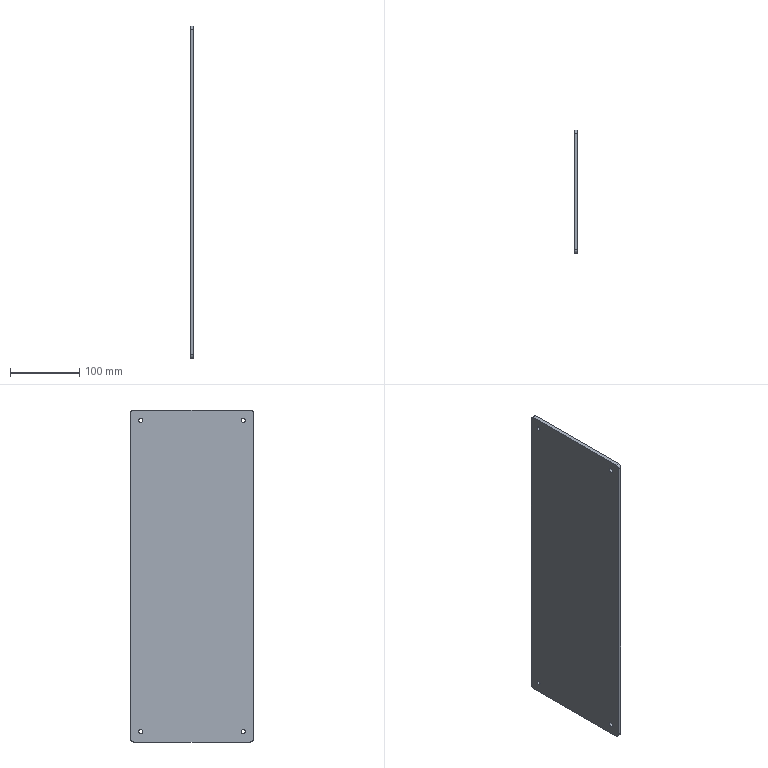Part | SolidWorks | features Extrusion 1, Fillet 1, ICE 1 | 1 solid | 18 faces | box 5 x 178 x 480 mm | volume 426527 mm3 | cylinder 12 | plane 6 | commonest cylinder face diameters 6 x8 10 x4
STEP:
#1=CARTESIAN_POINT('',(0.,-74.,-222.));
#2=VERTEX_POINT('',#1);
#3=CARTESIAN_POINT('',(0.,-74.,-228.));
#4=VERTEX_POINT('',#3);
#5=CARTESIAN_POINT('',(0.,-74.,-225.));
#6=DIRECTION('',(1.,0.,0.));
#7=DIRECTION('',(0.,0.,-1.));
#8=AXIS2_PLACEMENT_3D('',#5,#6,#7);
#9=CIRCLE('',#8,3.);
#10=EDGE_CURVE('',#2,#4,#9,.T.);
#11=ORIENTED_EDGE('',*,*,#10,.F.);
#12=CARTESIAN_POINT('',(5.,-74.,-222.));
#13=VERTEX_POINT('',#12);
#14=CARTESIAN_POINT('',(0.,-74.,-222.));
#15=DIRECTION('',(1.,0.,0.));
#16=VECTOR('',#15,1000.);
#17=LINE('',#14,#16);
#18=EDGE_CURVE('',#2,#13,#17,.T.);
#19=ORIENTED_EDGE('',*,*,#18,.T.);
#20=CARTESIAN_POINT('',(5.,-74.,-228.));
#21=VERTEX_POINT('',#20);
#22=CARTESIAN_POINT('',(5.,-74.,-225.));
#23=DIRECTION('',(1.,0.,0.));
#24=DIRECTION('',(0.,0.,-1.));
#25=AXIS2_PLACEMENT_3D('',#22,#23,#24);
#26=CIRCLE('',#25,3.);
#27=EDGE_CURVE('',#13,#21,#26,.T.);
#28=ORIENTED_EDGE('',*,*,#27,.T.);
#29=CARTESIAN_POINT('',(0.,-74.,-228.));
#30=DIRECTION('',(1.,0.,0.));
#31=VECTOR('',#30,1000.);
#32=LINE('',#29,#31);
#33=EDGE_CURVE('',#4,#21,#32,.T.);
#34=ORIENTED_EDGE('',*,*,#33,.F.);
#35=EDGE_LOOP('',(#11,#19,#28,#34));
#36=FACE_OUTER_BOUND('',#35,.T.);
#37=CARTESIAN_POINT('',(0.,-74.,-225.));
#38=DIRECTION('',(1.,0.,0.));
#39=DIRECTION('',(0.,0.,-1.));
#40=AXIS2_PLACEMENT_3D('',#37,#38,#39);
#41=CYLINDRICAL_SURFACE('',#40,3.);
#42=ADVANCED_FACE('',(#36),#41,.F.);
#43=CARTESIAN_POINT('',(0.,-74.,228.));
#44=VERTEX_POINT('',#43);
#45=CARTESIAN_POINT('',(0.,-74.,222.));
#46=VERTEX_POINT('',#45);
#47=CARTESIAN_POINT('',(0.,-74.,225.));
#48=DIRECTION('',(1.,0.,0.));
#49=DIRECTION('',(0.,0.,-1.));
#50=AXIS2_PLACEMENT_3D('',#47,#48,#49);
#51=CIRCLE('',#50,3.);
#52=EDGE_CURVE('',#44,#46,#51,.T.);
#53=ORIENTED_EDGE('',*,*,#52,.F.);
#54=CARTESIAN_POINT('',(5.,-74.,228.));
#55=VERTEX_POINT('',#54);
#56=CARTESIAN_POINT('',(0.,-74.,228.));
#57=DIRECTION('',(1.,0.,0.));
#58=VECTOR('',#57,1000.);
#59=LINE('',#56,#58);
#60=EDGE_CURVE('',#44,#55,#59,.T.);
#61=ORIENTED_EDGE('',*,*,#60,.T.);
#62=CARTESIAN_POINT('',(5.,-74.,222.));
#63=VERTEX_POINT('',#62);
#64=CARTESIAN_POINT('',(5.,-74.,225.));
#65=DIRECTION('',(1.,0.,0.));
#66=DIRECTION('',(0.,0.,-1.));
#67=AXIS2_PLACEMENT_3D('',#64,#65,#66);
#68=CIRCLE('',#67,3.);
#69=EDGE_CURVE('',#55,#63,#68,.T.);
#70=ORIENTED_EDGE('',*,*,#69,.T.);
#71=CARTESIAN_POINT('',(0.,-74.,222.));
#72=DIRECTION('',(1.,0.,0.));
#73=VECTOR('',#72,1000.);
#74=LINE('',#71,#73);
#75=EDGE_CURVE('',#46,#63,#74,.T.);
#76=ORIENTED_EDGE('',*,*,#75,.F.);
#77=EDGE_LOOP('',(#53,#61,#70,#76));
#78=FACE_OUTER_BOUND('',#77,.T.);
#79=CARTESIAN_POINT('',(0.,-74.,225.));
#80=DIRECTION('',(1.,0.,0.));
#81=DIRECTION('',(0.,0.,-1.));
#82=AXIS2_PLACEMENT_3D('',#79,#80,#81);
#83=CYLINDRICAL_SURFACE('',#82,3.);
#84=ADVANCED_FACE('',(#78),#83,.F.);
#85=CARTESIAN_POINT('',(0.,74.,-222.));
#86=VERTEX_POINT('',#85);
#87=CARTESIAN_POINT('',(0.,74.,-228.));
#88=VERTEX_POINT('',#87);
#89=CARTESIAN_POINT('',(0.,74.,-225.));
#90=DIRECTION('',(1.,0.,0.));
#91=DIRECTION('',(0.,0.,-1.));
#92=AXIS2_PLACEMENT_3D('',#89,#90,#91);
#93=CIRCLE('',#92,3.);
#94=EDGE_CURVE('',#86,#88,#93,.T.);
#95=ORIENTED_EDGE('',*,*,#94,.F.);
#96=CARTESIAN_POINT('',(5.,74.,-222.));
#97=VERTEX_POINT('',#96);
#98=CARTESIAN_POINT('',(0.,74.,-222.));
#99=DIRECTION('',(1.,0.,0.));
#100=VECTOR('',#99,1000.);
#101=LINE('',#98,#100);
#102=EDGE_CURVE('',#86,#97,#101,.T.);
#103=ORIENTED_EDGE('',*,*,#102,.T.);
#104=CARTESIAN_POINT('',(5.,74.,-228.));
#105=VERTEX_POINT('',#104);
#106=CARTESIAN_POINT('',(5.,74.,-225.));
#107=DIRECTION('',(1.,0.,0.));
#108=DIRECTION('',(0.,0.,-1.));
#109=AXIS2_PLACEMENT_3D('',#106,#107,#108);
#110=CIRCLE('',#109,3.);
#111=EDGE_CURVE('',#97,#105,#110,.T.);
#112=ORIENTED_EDGE('',*,*,#111,.T.);
#113=CARTESIAN_POINT('',(0.,74.,-228.));
#114=DIRECTION('',(1.,0.,0.));
#115=VECTOR('',#114,1000.);
#116=LINE('',#113,#115);
#117=EDGE_CURVE('',#88,#105,#116,.T.);
#118=ORIENTED_EDGE('',*,*,#117,.F.);
#119=EDGE_LOOP('',(#95,#103,#112,#118));
#120=FACE_OUTER_BOUND('',#119,.T.);
#121=CARTESIAN_POINT('',(0.,74.,-225.));
#122=DIRECTION('',(1.,0.,0.));
#123=DIRECTION('',(0.,0.,-1.));
#124=AXIS2_PLACEMENT_3D('',#121,#122,#123);
#125=CYLINDRICAL_SURFACE('',#124,3.);
#126=ADVANCED_FACE('',(#120),#125,.F.);
#127=CARTESIAN_POINT('',(0.,74.,228.));
#128=VERTEX_POINT('',#127);
#129=CARTESIAN_POINT('',(0.,74.,222.));
#130=VERTEX_POINT('',#129);
#131=CARTESIAN_POINT('',(0.,74.,225.));
#132=DIRECTION('',(1.,0.,0.));
#133=DIRECTION('',(0.,0.,-1.));
#134=AXIS2_PLACEMENT_3D('',#131,#132,#133);
#135=CIRCLE('',#134,3.);
#136=EDGE_CURVE('',#128,#130,#135,.T.);
#137=ORIENTED_EDGE('',*,*,#136,.F.);
#138=CARTESIAN_POINT('',(5.,74.,228.));
#139=VERTEX_POINT('',#138);
#140=CARTESIAN_POINT('',(0.,74.,228.));
#141=DIRECTION('',(1.,0.,0.));
#142=VECTOR('',#141,1000.);
#143=LINE('',#140,#142);
#144=EDGE_CURVE('',#128,#139,#143,.T.);
#145=ORIENTED_EDGE('',*,*,#144,.T.);
#146=CARTESIAN_POINT('',(5.,74.,222.));
#147=VERTEX_POINT('',#146);
#148=CARTESIAN_POINT('',(5.,74.,225.));
#149=DIRECTION('',(1.,0.,0.));
#150=DIRECTION('',(0.,0.,-1.));
#151=AXIS2_PLACEMENT_3D('',#148,#149,#150);
#152=CIRCLE('',#151,3.);
#153=EDGE_CURVE('',#139,#147,#152,.T.);
#154=ORIENTED_EDGE('',*,*,#153,.T.);
#155=CARTESIAN_POINT('',(0.,74.,222.));
#156=DIRECTION('',(1.,0.,0.));
#157=VECTOR('',#156,1000.);
#158=LINE('',#155,#157);
#159=EDGE_CURVE('',#130,#147,#158,.T.);
#160=ORIENTED_EDGE('',*,*,#159,.F.);
#161=EDGE_LOOP('',(#137,#145,#154,#160));
#162=FACE_OUTER_BOUND('',#161,.T.);
#163=CARTESIAN_POINT('',(0.,74.,225.));
#164=DIRECTION('',(1.,0.,0.));
#165=DIRECTION('',(0.,0.,-1.));
#166=AXIS2_PLACEMENT_3D('',#163,#164,#165);
#167=CYLINDRICAL_SURFACE('',#166,3.);
#168=ADVANCED_FACE('',(#162),#167,.F.);
#169=CARTESIAN_POINT('',(0.,84.,240.));
#170=VERTEX_POINT('',#169);
#171=CARTESIAN_POINT('',(0.,-84.,240.));
#172=VERTEX_POINT('',#171);
#173=CARTESIAN_POINT('',(0.,89.,240.));
#174=DIRECTION('',(0.,-1.,0.));
#175=VECTOR('',#174,1000.);
#176=LINE('',#173,#175);
#177=EDGE_CURVE('',#170,#172,#176,.T.);
#178=ORIENTED_EDGE('',*,*,#177,.T.);
#179=CARTESIAN_POINT('',(5.,-84.,240.));
#180=VERTEX_POINT('',#179);
#181=CARTESIAN_POINT('',(5.,-84.,240.));
#182=DIRECTION('',(1.,0.,0.));
#183=VECTOR('',#182,1000.);
#184=LINE('',#181,#183);
#185=EDGE_CURVE('',#172,#180,#184,.T.);
#186=ORIENTED_EDGE('',*,*,#185,.T.);
#187=CARTESIAN_POINT('',(5.,84.,240.));
#188=VERTEX_POINT('',#187);
#189=CARTESIAN_POINT('',(5.,89.,240.));
#190=DIRECTION('',(0.,-1.,0.));
#191=VECTOR('',#190,1000.);
#192=LINE('',#189,#191);
#193=EDGE_CURVE('',#188,#180,#192,.T.);
#194=ORIENTED_EDGE('',*,*,#193,.F.);
#195=CARTESIAN_POINT('',(5.,84.,240.));
#196=DIRECTION('',(-1.,0.,0.));
#197=VECTOR('',#196,1000.);
#198=LINE('',#195,#197);
#199=EDGE_CURVE('',#188,#170,#198,.T.);
#200=ORIENTED_EDGE('',*,*,#199,.T.);
#201=EDGE_LOOP('',(#178,#186,#194,#200));
#202=FACE_OUTER_BOUND('',#201,.T.);
#203=CARTESIAN_POINT('',(5.,89.,240.));
#204=DIRECTION('',(0.,0.,-1.));
#205=DIRECTION('',(-1.,0.,0.));
#206=AXIS2_PLACEMENT_3D('',#203,#204,#205);
#207=PLANE('',#206);
#208=ADVANCED_FACE('',(#202),#207,.F.);
#209=CARTESIAN_POINT('',(5.,-89.,235.));
#210=VERTEX_POINT('',#209);
#211=CARTESIAN_POINT('',(5.,-89.,-235.));
#212=VERTEX_POINT('',#211);
#213=CARTESIAN_POINT('',(5.,-89.,240.));
#214=DIRECTION('',(0.,0.,-1.));
#215=VECTOR('',#214,1000.);
#216=LINE('',#213,#215);
#217=EDGE_CURVE('',#210,#212,#216,.T.);
#218=ORIENTED_EDGE('',*,*,#217,.F.);
#219=CARTESIAN_POINT('',(0.,-89.,235.));
#220=VERTEX_POINT('',#219);
#221=CARTESIAN_POINT('',(5.,-89.,235.));
#222=DIRECTION('',(-1.,0.,0.));
#223=VECTOR('',#222,1000.);
#224=LINE('',#221,#223);
#225=EDGE_CURVE('',#210,#220,#224,.T.);
#226=ORIENTED_EDGE('',*,*,#225,.T.);
#227=CARTESIAN_POINT('',(0.,-89.,-235.));
#228=VERTEX_POINT('',#227);
#229=CARTESIAN_POINT('',(0.,-89.,240.));
#230=DIRECTION('',(0.,0.,-1.));
#231=VECTOR('',#230,1000.);
#232=LINE('',#229,#231);
#233=EDGE_CURVE('',#220,#228,#232,.T.);
#234=ORIENTED_EDGE('',*,*,#233,.T.);
#235=CARTESIAN_POINT('',(5.,-89.,-235.));
#236=DIRECTION('',(1.,0.,0.));
#237=VECTOR('',#236,1000.);
#238=LINE('',#235,#237);
#239=EDGE_CURVE('',#228,#212,#238,.T.);
#240=ORIENTED_EDGE('',*,*,#239,.T.);
#241=EDGE_LOOP('',(#218,#226,#234,#240));
#242=FACE_OUTER_BOUND('',#241,.T.);
#243=CARTESIAN_POINT('',(5.,-89.,240.));
#244=DIRECTION('',(0.,1.,0.));
#245=DIRECTION('',(0.,0.,1.));
#246=AXIS2_PLACEMENT_3D('',#243,#244,#245);
#247=PLANE('',#246);
#248=ADVANCED_FACE('',(#242),#247,.F.);
#249=CARTESIAN_POINT('',(5.,-84.,-240.));
#250=VERTEX_POINT('',#249);
#251=CARTESIAN_POINT('',(5.,84.,-240.));
#252=VERTEX_POINT('',#251);
#253=CARTESIAN_POINT('',(5.,89.,-240.));
#254=DIRECTION('',(0.,1.,0.));
#255=VECTOR('',#254,1000.);
#256=LINE('',#253,#255);
#257=EDGE_CURVE('',#250,#252,#256,.T.);
#258=ORIENTED_EDGE('',*,*,#257,.F.);
#259=CARTESIAN_POINT('',(0.,-84.,-240.));
#260=VERTEX_POINT('',#259);
#261=CARTESIAN_POINT('',(5.,-84.,-240.));
#262=DIRECTION('',(-1.,0.,0.));
#263=VECTOR('',#262,1000.);
#264=LINE('',#261,#263);
#265=EDGE_CURVE('',#250,#260,#264,.T.);
#266=ORIENTED_EDGE('',*,*,#265,.T.);
#267=CARTESIAN_POINT('',(0.,84.,-240.));
#268=VERTEX_POINT('',#267);
#269=CARTESIAN_POINT('',(0.,89.,-240.));
#270=DIRECTION('',(0.,1.,0.));
#271=VECTOR('',#270,1000.);
#272=LINE('',#269,#271);
#273=EDGE_CURVE('',#260,#268,#272,.T.);
#274=ORIENTED_EDGE('',*,*,#273,.T.);
#275=CARTESIAN_POINT('',(5.,84.,-240.));
#276=DIRECTION('',(1.,0.,0.));
#277=VECTOR('',#276,1000.);
#278=LINE('',#275,#277);
#279=EDGE_CURVE('',#268,#252,#278,.T.);
#280=ORIENTED_EDGE('',*,*,#279,.T.);
#281=EDGE_LOOP('',(#258,#266,#274,#280));
#282=FACE_OUTER_BOUND('',#281,.T.);
#283=CARTESIAN_POINT('',(5.,89.,-240.));
#284=DIRECTION('',(0.,0.,1.));
#285=DIRECTION('',(1.,0.,0.));
#286=AXIS2_PLACEMENT_3D('',#283,#284,#285);
#287=PLANE('',#286);
#288=ADVANCED_FACE('',(#282),#287,.F.);
#289=CARTESIAN_POINT('',(5.,89.,-235.));
#290=VERTEX_POINT('',#289);
#291=CARTESIAN_POINT('',(5.,89.,235.));
#292=VERTEX_POINT('',#291);
#293=CARTESIAN_POINT('',(5.,89.,240.));
#294=DIRECTION('',(0.,0.,1.));
#295=VECTOR('',#294,1000.);
#296=LINE('',#293,#295);
#297=EDGE_CURVE('',#290,#292,#296,.T.);
#298=ORIENTED_EDGE('',*,*,#297,.F.);
#299=CARTESIAN_POINT('',(0.,89.,-235.));
#300=VERTEX_POINT('',#299);
#301=CARTESIAN_POINT('',(5.,89.,-235.));
#302=DIRECTION('',(-1.,0.,0.));
#303=VECTOR('',#302,1000.);
#304=LINE('',#301,#303);
#305=EDGE_CURVE('',#290,#300,#304,.T.);
#306=ORIENTED_EDGE('',*,*,#305,.T.);
#307=CARTESIAN_POINT('',(0.,89.,235.));
#308=VERTEX_POINT('',#307);
#309=CARTESIAN_POINT('',(0.,89.,240.));
#310=DIRECTION('',(0.,0.,1.));
#311=VECTOR('',#310,1000.);
#312=LINE('',#309,#311);
#313=EDGE_CURVE('',#300,#308,#312,.T.);
#314=ORIENTED_EDGE('',*,*,#313,.T.);
#315=CARTESIAN_POINT('',(5.,89.,235.));
#316=DIRECTION('',(1.,0.,0.));
#317=VECTOR('',#316,1000.);
#318=LINE('',#315,#317);
#319=EDGE_CURVE('',#308,#292,#318,.T.);
#320=ORIENTED_EDGE('',*,*,#319,.T.);
#321=EDGE_LOOP('',(#298,#306,#314,#320));
#322=FACE_OUTER_BOUND('',#321,.T.);
#323=CARTESIAN_POINT('',(5.,89.,240.));
#324=DIRECTION('',(0.,-1.,0.));
#325=DIRECTION('',(0.,0.,-1.));
#326=AXIS2_PLACEMENT_3D('',#323,#324,#325);
#327=PLANE('',#326);
#328=ADVANCED_FACE('',(#322),#327,.F.);
#329=CARTESIAN_POINT('',(5.,-74.,-225.));
#330=DIRECTION('',(1.,0.,0.));
#331=DIRECTION('',(0.,0.,-1.));
#332=AXIS2_PLACEMENT_3D('',#329,#330,#331);
#333=CIRCLE('',#332,3.);
#334=EDGE_CURVE('',#21,#13,#333,.T.);
#335=ORIENTED_EDGE('',*,*,#334,.F.);
#336=ORIENTED_EDGE('',*,*,#27,.F.);
#337=EDGE_LOOP('',(#335,#336));
#338=FACE_BOUND('',#337,.T.);
#339=CARTESIAN_POINT('',(5.,-74.,225.));
#340=DIRECTION('',(1.,0.,0.));
#341=DIRECTION('',(0.,0.,-1.));
#342=AXIS2_PLACEMENT_3D('',#339,#340,#341);
#343=CIRCLE('',#342,3.);
#344=EDGE_CURVE('',#63,#55,#343,.T.);
#345=ORIENTED_EDGE('',*,*,#344,.F.);
#346=ORIENTED_EDGE('',*,*,#69,.F.);
#347=EDGE_LOOP('',(#345,#346));
#348=FACE_BOUND('',#347,.T.);
#349=CARTESIAN_POINT('',(5.,74.,-225.));
#350=DIRECTION('',(1.,0.,0.));
#351=DIRECTION('',(0.,0.,-1.));
#352=AXIS2_PLACEMENT_3D('',#349,#350,#351);
#353=CIRCLE('',#352,3.);
#354=EDGE_CURVE('',#105,#97,#353,.T.);
#355=ORIENTED_EDGE('',*,*,#354,.F.);
#356=ORIENTED_EDGE('',*,*,#111,.F.);
#357=EDGE_LOOP('',(#355,#356));
#358=FACE_BOUND('',#357,.T.);
#359=CARTESIAN_POINT('',(5.,74.,225.));
#360=DIRECTION('',(1.,0.,0.));
#361=DIRECTION('',(0.,0.,-1.));
#362=AXIS2_PLACEMENT_3D('',#359,#360,#361);
#363=CIRCLE('',#362,3.);
#364=EDGE_CURVE('',#147,#139,#363,.T.);
#365=ORIENTED_EDGE('',*,*,#364,.F.);
#366=ORIENTED_EDGE('',*,*,#153,.F.);
#367=EDGE_LOOP('',(#365,#366));
#368=FACE_BOUND('',#367,.T.);
#369=ORIENTED_EDGE('',*,*,#193,.T.);
#370=CARTESIAN_POINT('',(5.,-84.,235.));
#371=DIRECTION('',(1.,0.,0.));
#372=DIRECTION('',(0.,0.,-1.));
#373=AXIS2_PLACEMENT_3D('',#370,#371,#372);
#374=CIRCLE('',#373,5.);
#375=EDGE_CURVE('',#180,#210,#374,.T.);
#376=ORIENTED_EDGE('',*,*,#375,.T.);
#377=ORIENTED_EDGE('',*,*,#217,.T.);
#378=CARTESIAN_POINT('',(5.,-84.,-235.));
#379=DIRECTION('',(1.,0.,0.));
#380=DIRECTION('',(0.,0.,-1.));
#381=AXIS2_PLACEMENT_3D('',#378,#379,#380);
#382=CIRCLE('',#381,5.);
#383=EDGE_CURVE('',#212,#250,#382,.T.);
#384=ORIENTED_EDGE('',*,*,#383,.T.);
#385=ORIENTED_EDGE('',*,*,#257,.T.);
#386=CARTESIAN_POINT('',(5.,84.,-235.));
#387=DIRECTION('',(1.,0.,0.));
#388=DIRECTION('',(0.,0.,-1.));
#389=AXIS2_PLACEMENT_3D('',#386,#387,#388);
#390=CIRCLE('',#389,5.);
#391=EDGE_CURVE('',#252,#290,#390,.T.);
#392=ORIENTED_EDGE('',*,*,#391,.T.);
#393=ORIENTED_EDGE('',*,*,#297,.T.);
#394=CARTESIAN_POINT('',(5.,84.,235.));
#395=DIRECTION('',(1.,0.,0.));
#396=DIRECTION('',(0.,0.,-1.));
#397=AXIS2_PLACEMENT_3D('',#394,#395,#396);
#398=CIRCLE('',#397,5.);
#399=EDGE_CURVE('',#292,#188,#398,.T.);
#400=ORIENTED_EDGE('',*,*,#399,.T.);
#401=EDGE_LOOP('',(#369,#376,#377,#384,#385,#392,#393,#400));
#402=FACE_OUTER_BOUND('',#401,.T.);
#403=CARTESIAN_POINT('',(5.,0.,0.));
#404=DIRECTION('',(1.,0.,0.));
#405=DIRECTION('',(0.,0.,-1.));
#406=AXIS2_PLACEMENT_3D('',#403,#404,#405);
#407=PLANE('',#406);
#408=ADVANCED_FACE('',(#338,#348,#358,#368,#402),#407,.T.);
#409=CARTESIAN_POINT('',(0.,-74.,-225.));
#410=DIRECTION('',(1.,0.,0.));
#411=DIRECTION('',(0.,0.,-1.));
#412=AXIS2_PLACEMENT_3D('',#409,#410,#411);
#413=CIRCLE('',#412,3.);
#414=EDGE_CURVE('',#4,#2,#413,.T.);
#415=ORIENTED_EDGE('',*,*,#414,.T.);
#416=ORIENTED_EDGE('',*,*,#10,.T.);
#417=EDGE_LOOP('',(#415,#416));
#418=FACE_BOUND('',#417,.T.);
#419=CARTESIAN_POINT('',(0.,-74.,225.));
#420=DIRECTION('',(1.,0.,0.));
#421=DIRECTION('',(0.,0.,-1.));
#422=AXIS2_PLACEMENT_3D('',#419,#420,#421);
#423=CIRCLE('',#422,3.);
#424=EDGE_CURVE('',#46,#44,#423,.T.);
#425=ORIENTED_EDGE('',*,*,#424,.T.);
#426=ORIENTED_EDGE('',*,*,#52,.T.);
#427=EDGE_LOOP('',(#425,#426));
#428=FACE_BOUND('',#427,.T.);
#429=CARTESIAN_POINT('',(0.,74.,-225.));
#430=DIRECTION('',(1.,0.,0.));
#431=DIRECTION('',(0.,0.,-1.));
#432=AXIS2_PLACEMENT_3D('',#429,#430,#431);
#433=CIRCLE('',#432,3.);
#434=EDGE_CURVE('',#88,#86,#433,.T.);
#435=ORIENTED_EDGE('',*,*,#434,.T.);
#436=ORIENTED_EDGE('',*,*,#94,.T.);
#437=EDGE_LOOP('',(#435,#436));
#438=FACE_BOUND('',#437,.T.);
#439=CARTESIAN_POINT('',(0.,74.,225.));
#440=DIRECTION('',(1.,0.,0.));
#441=DIRECTION('',(0.,0.,-1.));
#442=AXIS2_PLACEMENT_3D('',#439,#440,#441);
#443=CIRCLE('',#442,3.);
#444=EDGE_CURVE('',#130,#128,#443,.T.);
#445=ORIENTED_EDGE('',*,*,#444,.T.);
#446=ORIENTED_EDGE('',*,*,#136,.T.);
#447=EDGE_LOOP('',(#445,#446));
#448=FACE_BOUND('',#447,.T.);
#449=ORIENTED_EDGE('',*,*,#233,.F.);
#450=CARTESIAN_POINT('',(0.,-84.,235.));
#451=DIRECTION('',(-1.,0.,0.));
#452=DIRECTION('',(0.,0.,-1.));
#453=AXIS2_PLACEMENT_3D('',#450,#451,#452);
#454=CIRCLE('',#453,5.);
#455=EDGE_CURVE('',#220,#172,#454,.T.);
#456=ORIENTED_EDGE('',*,*,#455,.T.);
#457=ORIENTED_EDGE('',*,*,#177,.F.);
#458=CARTESIAN_POINT('',(0.,84.,235.));
#459=DIRECTION('',(-1.,0.,0.));
#460=DIRECTION('',(0.,0.,-1.));
#461=AXIS2_PLACEMENT_3D('',#458,#459,#460);
#462=CIRCLE('',#461,5.);
#463=EDGE_CURVE('',#170,#308,#462,.T.);
#464=ORIENTED_EDGE('',*,*,#463,.T.);
#465=ORIENTED_EDGE('',*,*,#313,.F.);
#466=CARTESIAN_POINT('',(0.,84.,-235.));
#467=DIRECTION('',(-1.,0.,0.));
#468=DIRECTION('',(0.,0.,-1.));
#469=AXIS2_PLACEMENT_3D('',#466,#467,#468);
#470=CIRCLE('',#469,5.);
#471=EDGE_CURVE('',#300,#268,#470,.T.);
#472=ORIENTED_EDGE('',*,*,#471,.T.);
#473=ORIENTED_EDGE('',*,*,#273,.F.);
#474=CARTESIAN_POINT('',(0.,-84.,-235.));
#475=DIRECTION('',(-1.,0.,0.));
#476=DIRECTION('',(0.,0.,-1.));
#477=AXIS2_PLACEMENT_3D('',#474,#475,#476);
#478=CIRCLE('',#477,5.);
#479=EDGE_CURVE('',#260,#228,#478,.T.);
#480=ORIENTED_EDGE('',*,*,#479,.T.);
#481=EDGE_LOOP('',(#449,#456,#457,#464,#465,#472,#473,#480));
#482=FACE_OUTER_BOUND('',#481,.T.);
#483=CARTESIAN_POINT('',(0.,0.,0.));
#484=DIRECTION('',(1.,0.,0.));
#485=DIRECTION('',(0.,0.,-1.));
#486=AXIS2_PLACEMENT_3D('',#483,#484,#485);
#487=PLANE('',#486);
#488=ADVANCED_FACE('',(#418,#428,#438,#448,#482),#487,.F.);
#489=ORIENTED_EDGE('',*,*,#144,.F.);
#490=ORIENTED_EDGE('',*,*,#444,.F.);
#491=ORIENTED_EDGE('',*,*,#159,.T.);
#492=ORIENTED_EDGE('',*,*,#364,.T.);
#493=EDGE_LOOP('',(#489,#490,#491,#492));
#494=FACE_OUTER_BOUND('',#493,.T.);
#495=CARTESIAN_POINT('',(0.,74.,225.));
#496=DIRECTION('',(1.,0.,0.));
#497=DIRECTION('',(0.,0.,-1.));
#498=AXIS2_PLACEMENT_3D('',#495,#496,#497);
#499=CYLINDRICAL_SURFACE('',#498,3.);
#500=ADVANCED_FACE('',(#494),#499,.F.);
#501=ORIENTED_EDGE('',*,*,#102,.F.);
#502=ORIENTED_EDGE('',*,*,#434,.F.);
#503=ORIENTED_EDGE('',*,*,#117,.T.);
#504=ORIENTED_EDGE('',*,*,#354,.T.);
#505=EDGE_LOOP('',(#501,#502,#503,#504));
#506=FACE_OUTER_BOUND('',#505,.T.);
#507=CARTESIAN_POINT('',(0.,74.,-225.));
#508=DIRECTION('',(1.,0.,0.));
#509=DIRECTION('',(0.,0.,-1.));
#510=AXIS2_PLACEMENT_3D('',#507,#508,#509);
#511=CYLINDRICAL_SURFACE('',#510,3.);
#512=ADVANCED_FACE('',(#506),#511,.F.);
#513=ORIENTED_EDGE('',*,*,#60,.F.);
#514=ORIENTED_EDGE('',*,*,#424,.F.);
#515=ORIENTED_EDGE('',*,*,#75,.T.);
#516=ORIENTED_EDGE('',*,*,#344,.T.);
#517=EDGE_LOOP('',(#513,#514,#515,#516));
#518=FACE_OUTER_BOUND('',#517,.T.);
#519=CARTESIAN_POINT('',(0.,-74.,225.));
#520=DIRECTION('',(1.,0.,0.));
#521=DIRECTION('',(0.,0.,-1.));
#522=AXIS2_PLACEMENT_3D('',#519,#520,#521);
#523=CYLINDRICAL_SURFACE('',#522,3.);
#524=ADVANCED_FACE('',(#518),#523,.F.);
#525=ORIENTED_EDGE('',*,*,#18,.F.);
#526=ORIENTED_EDGE('',*,*,#414,.F.);
#527=ORIENTED_EDGE('',*,*,#33,.T.);
#528=ORIENTED_EDGE('',*,*,#334,.T.);
#529=EDGE_LOOP('',(#525,#526,#527,#528));
#530=FACE_OUTER_BOUND('',#529,.T.);
#531=CARTESIAN_POINT('',(0.,-74.,-225.));
#532=DIRECTION('',(1.,0.,0.));
#533=DIRECTION('',(0.,0.,-1.));
#534=AXIS2_PLACEMENT_3D('',#531,#532,#533);
#535=CYLINDRICAL_SURFACE('',#534,3.);
#536=ADVANCED_FACE('',(#530),#535,.F.);
#537=ORIENTED_EDGE('',*,*,#375,.F.);
#538=ORIENTED_EDGE('',*,*,#185,.F.);
#539=ORIENTED_EDGE('',*,*,#455,.F.);
#540=ORIENTED_EDGE('',*,*,#225,.F.);
#541=EDGE_LOOP('',(#537,#538,#539,#540));
#542=FACE_OUTER_BOUND('',#541,.T.);
#543=CARTESIAN_POINT('',(5.,-84.,235.));
#544=DIRECTION('',(-1.,0.,0.));
#545=DIRECTION('',(0.,0.,1.));
#546=AXIS2_PLACEMENT_3D('',#543,#544,#545);
#547=CYLINDRICAL_SURFACE('',#546,5.);
#548=ADVANCED_FACE('',(#542),#547,.T.);
#549=ORIENTED_EDGE('',*,*,#383,.F.);
#550=ORIENTED_EDGE('',*,*,#239,.F.);
#551=ORIENTED_EDGE('',*,*,#479,.F.);
#552=ORIENTED_EDGE('',*,*,#265,.F.);
#553=EDGE_LOOP('',(#549,#550,#551,#552));
#554=FACE_OUTER_BOUND('',#553,.T.);
#555=CARTESIAN_POINT('',(5.,-84.,-235.));
#556=DIRECTION('',(-1.,0.,0.));
#557=DIRECTION('',(0.,0.,1.));
#558=AXIS2_PLACEMENT_3D('',#555,#556,#557);
#559=CYLINDRICAL_SURFACE('',#558,5.);
#560=ADVANCED_FACE('',(#554),#559,.T.);
#561=ORIENTED_EDGE('',*,*,#391,.F.);
#562=ORIENTED_EDGE('',*,*,#279,.F.);
#563=ORIENTED_EDGE('',*,*,#471,.F.);
#564=ORIENTED_EDGE('',*,*,#305,.F.);
#565=EDGE_LOOP('',(#561,#562,#563,#564));
#566=FACE_OUTER_BOUND('',#565,.T.);
#567=CARTESIAN_POINT('',(5.,84.,-235.));
#568=DIRECTION('',(-1.,0.,0.));
#569=DIRECTION('',(0.,0.,1.));
#570=AXIS2_PLACEMENT_3D('',#567,#568,#569);
#571=CYLINDRICAL_SURFACE('',#570,5.);
#572=ADVANCED_FACE('',(#566),#571,.T.);
#573=ORIENTED_EDGE('',*,*,#399,.F.);
#574=ORIENTED_EDGE('',*,*,#319,.F.);
#575=ORIENTED_EDGE('',*,*,#463,.F.);
#576=ORIENTED_EDGE('',*,*,#199,.F.);
#577=EDGE_LOOP('',(#573,#574,#575,#576));
#578=FACE_OUTER_BOUND('',#577,.T.);
#579=CARTESIAN_POINT('',(5.,84.,235.));
#580=DIRECTION('',(-1.,0.,0.));
#581=DIRECTION('',(0.,0.,1.));
#582=AXIS2_PLACEMENT_3D('',#579,#580,#581);
#583=CYLINDRICAL_SURFACE('',#582,5.);
#584=ADVANCED_FACE('',(#578),#583,.T.);
#585=CLOSED_SHELL('',(#42,#84,#126,#168,#208,#248,#288,#328,#408,#488,#500,#512,#524,#536,#548,#560,#572,#584));
#586=MANIFOLD_SOLID_BREP('',#585);
#587=CARTESIAN_POINT('',(0.,0.,0.));
#588=DIRECTION('',(0.,0.,1.));
#589=DIRECTION('',(1.,0.,0.));
#590=AXIS2_PLACEMENT_3D('',#587,#588,#589);
#591=(LENGTH_UNIT()NAMED_UNIT(*)SI_UNIT(.MILLI.,.METRE.));
#592=UNCERTAINTY_MEASURE_WITH_UNIT(LENGTH_MEASURE(0.00001),#591,'','');
#593=(NAMED_UNIT(*)PLANE_ANGLE_UNIT()SI_UNIT($,.RADIAN.));
#594=(NAMED_UNIT(*)SI_UNIT($,.STERADIAN.)SOLID_ANGLE_UNIT());
#595=(GEOMETRIC_REPRESENTATION_CONTEXT(3)GLOBAL_UNCERTAINTY_ASSIGNED_CONTEXT((#592))GLOBAL_UNIT_ASSIGNED_CONTEXT((#591,#593,#594))REPRESENTATION_CONTEXT('',''));
#596=ADVANCED_BREP_SHAPE_REPRESENTATION('',(#586,#590),#595);